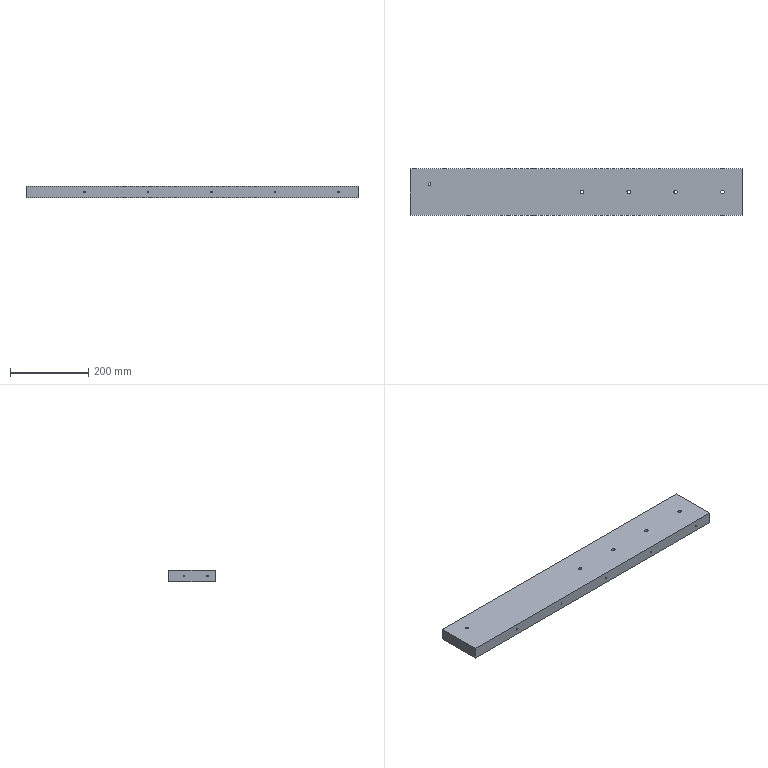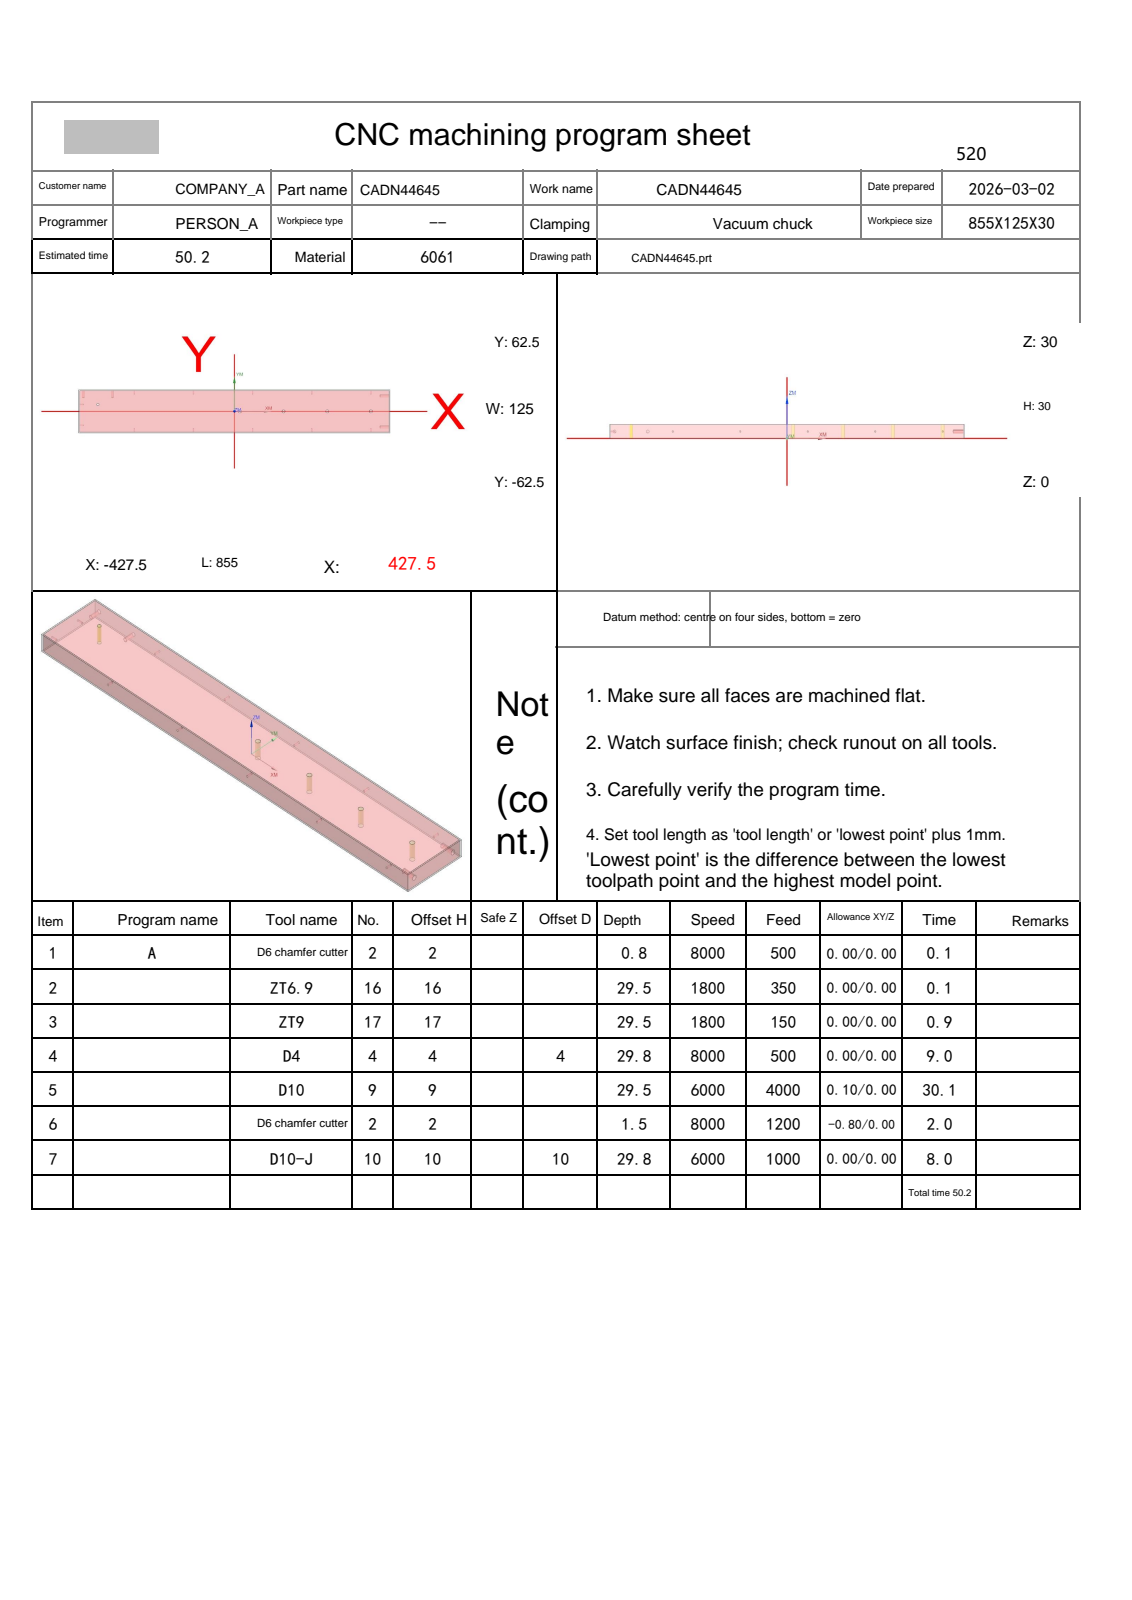NC program | NX | posted by the shop | part box 850 x 120 x 30 mm
Lines 1 to 1477 of 2164, first 1115 of 1475 lines:
%
O0001
(Machine time: 51.65 MIN)
(===Total Tool:6===)
(T2=D6 chamfer cutter   D=6.   R=0.   D-  H02 Z=28.5  )
(T16=ZT6.9  D=6.9  DR_a=120 D-  H16 Z=0.5   )
(T17=ZT9    D=9.   DR_a=118 D-  H17 Z=0.5   )
(T4=D4      D=4.   R=0.   D4  H04 Z=0.2   )
(T9=D10     D=10.  R=0.   D-  H09 Z=0.5   )
(T10=D10-J  D=10.  R=0.   D10 H10 Z=0.2   )
G80 G90 G17 G49 G40
G91 G28 Z0
M01
N1 T02 M06
(D6 chamfer cutter  D=6. R=0. H=02 ce=0.00 di=0.00)
G00 G90 G54 X-375. Y20. M03 S8000
G43 H02 Z80.
M08
G98 G81 X-375. Y20. Z29.2 R31. F500.
X15. Y0.0
X135.
X255.
X375.
G80
G00 Z80.
G91 G28 Z0.0
M05
M09
G91 G28 Z0.0
M01
N2 T16 M06
(ZT6.9 D=6.9 DR_a=120 H=16)
G00 G90 G54 X-375. Y20. M03 S1800
G43 H16 Z80.
M08
G98 G83 X-375. Y20. Z.5 R31. F350. Q3.
G80
G00 Z80.
G91 G28 Z0.0
M05
M09
G91 G28 Z0.0
M01
N3 T17 M06
(ZT9 D=9. DR_a=118 H=17)
G00 G90 G54 X375. Y0.0 M03 S1800
G43 H17 Z80.
M08
G98 G83 X375. Y0.0 Z.5 R31. F150. Q3.
X255.
X135.
X15.
G80
G00 Z80.
G91 G28 Z0.0
M05
M09
G91 G28 Z0.0
M01
N4 T04 M06
(D4  D=4. R=0. H=04 ce=0.00 di=0.00)
G00 G90 G54 X373.18 Y1.661 M03 S8000
G43 H04 Z80.
M08
Z30.5
G01 X373.119 Y1.601 Z30.496 F500.
X372.888 Y1.28 Z30.475
X372.71 Y.926 Z30.454
X372.592 Y.549 Z30.433
X372.535 Y.157 Z30.413
Y-.157 Z30.396
X372.592 Y-.549 Z30.375
X372.71 Y-.926 Z30.355
X372.888 Y-1.28 Z30.334
X373.119 Y-1.601 Z30.313
X373.399 Y-1.881 Z30.292
X373.72 Y-2.112 Z30.272
X374.074 Y-2.29 Z30.251
X374.451 Y-2.408 Z30.23
X374.843 Y-2.465 Z30.209
X375.157 Z30.193
X375.593 Y-2.398 Z30.17
X376.009 Y-2.254 Z30.147
X376.394 Y-2.039 Z30.124
X376.734 Y-1.759 Z30.101
X377.019 Y-1.423 Z30.078
X377.24 Y-1.041 Z30.054
X377.389 Y-.627 Z30.031
X377.462 Y-.192 Z30.008
X377.465 Y-.035 Z30.
G41 D04
X377.5 Y0.0
G03 X375. Y2.5 Z29.876 I-2.5 J0.0
X372.5 Y0.0 Z29.752 I0.0 J-2.5
X375. Y-2.5 Z29.628 I2.5 J0.0
X377.5 Y0.0 Z29.503 I0.0 J2.5
X375. Y2.5 Z29.379 I-2.5 J0.0
X372.5 Y0.0 Z29.255 I0.0 J-2.5
X375. Y-2.5 Z29.131 I2.5 J0.0
X377.5 Y0.0 Z29.007 I0.0 J2.5
X375. Y2.5 Z28.883 I-2.5 J0.0
X372.5 Y0.0 Z28.758 I0.0 J-2.5
X375. Y-2.5 Z28.634 I2.5 J0.0
X377.5 Y0.0 Z28.51 I0.0 J2.5
X375. Y2.5 Z28.386 I-2.5 J0.0
X372.5 Y0.0 Z28.262 I0.0 J-2.5
X375. Y-2.5 Z28.138 I2.5 J0.0
X377.5 Y0.0 Z28.013 I0.0 J2.5
X375. Y2.5 Z27.889 I-2.5 J0.0
X372.5 Y0.0 Z27.765 I0.0 J-2.5
X375. Y-2.5 Z27.641 I2.5 J0.0
X377.5 Y0.0 Z27.517 I0.0 J2.5
X375. Y2.5 Z27.393 I-2.5 J0.0
X372.5 Y0.0 Z27.268 I0.0 J-2.5
X375. Y-2.5 Z27.144 I2.5 J0.0
X377.5 Y0.0 Z27.02 I0.0 J2.5
X375. Y2.5 Z26.896 I-2.5 J0.0
X372.5 Y0.0 Z26.772 I0.0 J-2.5
X375. Y-2.5 Z26.648 I2.5 J0.0
X377.5 Y0.0 Z26.523 I0.0 J2.5
X375. Y2.5 Z26.399 I-2.5 J0.0
X372.5 Y0.0 Z26.275 I0.0 J-2.5
X375. Y-2.5 Z26.151 I2.5 J0.0
X377.5 Y0.0 Z26.027 I0.0 J2.5
X375. Y2.5 Z25.903 I-2.5 J0.0
X372.5 Y0.0 Z25.778 I0.0 J-2.5
X375. Y-2.5 Z25.654 I2.5 J0.0
X377.5 Y0.0 Z25.53 I0.0 J2.5
X375. Y2.5 Z25.406 I-2.5 J0.0
X372.5 Y0.0 Z25.282 I0.0 J-2.5
X375. Y-2.5 Z25.158 I2.5 J0.0
X377.5 Y0.0 Z25.033 I0.0 J2.5
X375. Y2.5 Z24.909 I-2.5 J0.0
X372.5 Y0.0 Z24.785 I0.0 J-2.5
X375. Y-2.5 Z24.661 I2.5 J0.0
X377.5 Y0.0 Z24.537 I0.0 J2.5
X375. Y2.5 Z24.413 I-2.5 J0.0
X372.5 Y0.0 Z24.288 I0.0 J-2.5
X375. Y-2.5 Z24.164 I2.5 J0.0
X377.5 Y0.0 Z24.04 I0.0 J2.5
X375. Y2.5 Z23.916 I-2.5 J0.0
X372.5 Y0.0 Z23.792 I0.0 J-2.5
X375. Y-2.5 Z23.668 I2.5 J0.0
X377.5 Y0.0 Z23.543 I0.0 J2.5
X375. Y2.5 Z23.419 I-2.5 J0.0
X372.5 Y0.0 Z23.295 I0.0 J-2.5
X375. Y-2.5 Z23.171 I2.5 J0.0
X377.5 Y0.0 Z23.047 I0.0 J2.5
X375. Y2.5 Z22.923 I-2.5 J0.0
X372.5 Y0.0 Z22.798 I0.0 J-2.5
X375. Y-2.5 Z22.674 I2.5 J0.0
X377.5 Y0.0 Z22.55 I0.0 J2.5
X375. Y2.5 Z22.426 I-2.5 J0.0
X372.5 Y0.0 Z22.302 I0.0 J-2.5
X375. Y-2.5 Z22.178 I2.5 J0.0
X377.5 Y0.0 Z22.053 I0.0 J2.5
X375. Y2.5 Z21.929 I-2.5 J0.0
X372.5 Y0.0 Z21.805 I0.0 J-2.5
X375. Y-2.5 Z21.681 I2.5 J0.0
X377.5 Y0.0 Z21.557 I0.0 J2.5
X375. Y2.5 Z21.433 I-2.5 J0.0
X372.5 Y0.0 Z21.308 I0.0 J-2.5
X375. Y-2.5 Z21.184 I2.5 J0.0
X377.5 Y0.0 Z21.06 I0.0 J2.5
X375. Y2.5 Z20.936 I-2.5 J0.0
X372.5 Y0.0 Z20.812 I0.0 J-2.5
X375. Y-2.5 Z20.688 I2.5 J0.0
X377.5 Y0.0 Z20.563 I0.0 J2.5
X375. Y2.5 Z20.439 I-2.5 J0.0
X372.5 Y0.0 Z20.315 I0.0 J-2.5
X375. Y-2.5 Z20.191 I2.5 J0.0
X377.5 Y0.0 Z20.067 I0.0 J2.5
X375. Y2.5 Z19.943 I-2.5 J0.0
X372.5 Y0.0 Z19.818 I0.0 J-2.5
X375. Y-2.5 Z19.694 I2.5 J0.0
X377.5 Y0.0 Z19.57 I0.0 J2.5
X375. Y2.5 Z19.446 I-2.5 J0.0
X372.5 Y0.0 Z19.322 I0.0 J-2.5
X375. Y-2.5 Z19.198 I2.5 J0.0
X377.5 Y0.0 Z19.073 I0.0 J2.5
X375. Y2.5 Z18.949 I-2.5 J0.0
X372.5 Y0.0 Z18.825 I0.0 J-2.5
X375. Y-2.5 Z18.701 I2.5 J0.0
X377.5 Y0.0 Z18.577 I0.0 J2.5
X375. Y2.5 Z18.453 I-2.5 J0.0
X372.5 Y0.0 Z18.328 I0.0 J-2.5
X375. Y-2.5 Z18.204 I2.5 J0.0
X377.5 Y0.0 Z18.08 I0.0 J2.5
X375. Y2.5 Z17.956 I-2.5 J0.0
X372.5 Y0.0 Z17.832 I0.0 J-2.5
X375. Y-2.5 Z17.708 I2.5 J0.0
X377.5 Y0.0 Z17.583 I0.0 J2.5
X375. Y2.5 Z17.459 I-2.5 J0.0
X372.5 Y0.0 Z17.335 I0.0 J-2.5
X375. Y-2.5 Z17.211 I2.5 J0.0
X377.5 Y0.0 Z17.087 I0.0 J2.5
X375. Y2.5 Z16.963 I-2.5 J0.0
X372.5 Y0.0 Z16.838 I0.0 J-2.5
X375. Y-2.5 Z16.714 I2.5 J0.0
X377.5 Y0.0 Z16.59 I0.0 J2.5
X375. Y2.5 Z16.466 I-2.5 J0.0
X372.5 Y0.0 Z16.342 I0.0 J-2.5
X375. Y-2.5 Z16.218 I2.5 J0.0
X377.5 Y0.0 Z16.093 I0.0 J2.5
X375. Y2.5 Z15.969 I-2.5 J0.0
X372.5 Y0.0 Z15.845 I0.0 J-2.5
X375. Y-2.5 Z15.721 I2.5 J0.0
X377.5 Y0.0 Z15.597 I0.0 J2.5
X375. Y2.5 Z15.473 I-2.5 J0.0
X372.5 Y0.0 Z15.348 I0.0 J-2.5
X375. Y-2.5 Z15.224 I2.5 J0.0
X377.5 Y0.0 Z15.1 I0.0 J2.5
X375. Y2.5 Z14.976 I-2.5 J0.0
X372.5 Y0.0 Z14.852 I0.0 J-2.5
X375. Y-2.5 Z14.728 I2.5 J0.0
X377.5 Y0.0 Z14.603 I0.0 J2.5
X375. Y2.5 Z14.479 I-2.5 J0.0
X372.5 Y0.0 Z14.355 I0.0 J-2.5
X375. Y-2.5 Z14.231 I2.5 J0.0
X377.5 Y0.0 Z14.107 I0.0 J2.5
X375. Y2.5 Z13.983 I-2.5 J0.0
X372.5 Y0.0 Z13.858 I0.0 J-2.5
X375. Y-2.5 Z13.734 I2.5 J0.0
X377.5 Y0.0 Z13.61 I0.0 J2.5
X375. Y2.5 Z13.486 I-2.5 J0.0
X372.5 Y0.0 Z13.362 I0.0 J-2.5
X375. Y-2.5 Z13.238 I2.5 J0.0
X377.5 Y0.0 Z13.113 I0.0 J2.5
X375. Y2.5 Z12.989 I-2.5 J0.0
X372.5 Y0.0 Z12.865 I0.0 J-2.5
X375. Y-2.5 Z12.741 I2.5 J0.0
X377.5 Y0.0 Z12.617 I0.0 J2.5
X375. Y2.5 Z12.493 I-2.5 J0.0
X372.5 Y0.0 Z12.368 I0.0 J-2.5
X375. Y-2.5 Z12.244 I2.5 J0.0
X377.5 Y0.0 Z12.12 I0.0 J2.5
X375. Y2.5 Z11.996 I-2.5 J0.0
X372.5 Y0.0 Z11.872 I0.0 J-2.5
X375. Y-2.5 Z11.748 I2.5 J0.0
X377.5 Y0.0 Z11.623 I0.0 J2.5
X375. Y2.5 Z11.499 I-2.5 J0.0
X372.5 Y0.0 Z11.375 I0.0 J-2.5
X375. Y-2.5 Z11.251 I2.5 J0.0
X377.5 Y0.0 Z11.127 I0.0 J2.5
X375. Y2.5 Z11.003 I-2.5 J0.0
X372.5 Y0.0 Z10.878 I0.0 J-2.5
X375. Y-2.5 Z10.754 I2.5 J0.0
X377.5 Y0.0 Z10.63 I0.0 J2.5
X375. Y2.5 Z10.506 I-2.5 J0.0
X372.5 Y0.0 Z10.382 I0.0 J-2.5
X375. Y-2.5 Z10.258 I2.5 J0.0
X377.5 Y0.0 Z10.133 I0.0 J2.5
X375. Y2.5 Z10.009 I-2.5 J0.0
X372.5 Y0.0 Z9.885 I0.0 J-2.5
X375. Y-2.5 Z9.761 I2.5 J0.0
X377.5 Y0.0 Z9.637 I0.0 J2.5
X375. Y2.5 Z9.513 I-2.5 J0.0
X372.5 Y0.0 Z9.388 I0.0 J-2.5
X375. Y-2.5 Z9.264 I2.5 J0.0
X377.5 Y0.0 Z9.14 I0.0 J2.5
X375. Y2.5 Z9.016 I-2.5 J0.0
X372.5 Y0.0 Z8.892 I0.0 J-2.5
X375. Y-2.5 Z8.768 I2.5 J0.0
X377.5 Y0.0 Z8.643 I0.0 J2.5
X375. Y2.5 Z8.519 I-2.5 J0.0
X372.5 Y0.0 Z8.395 I0.0 J-2.5
X375. Y-2.5 Z8.271 I2.5 J0.0
X377.5 Y0.0 Z8.147 I0.0 J2.5
X375. Y2.5 Z8.023 I-2.5 J0.0
X372.5 Y0.0 Z7.898 I0.0 J-2.5
X375. Y-2.5 Z7.774 I2.5 J0.0
X377.5 Y0.0 Z7.65 I0.0 J2.5
X375. Y2.5 Z7.526 I-2.5 J0.0
X372.5 Y0.0 Z7.402 I0.0 J-2.5
X375. Y-2.5 Z7.278 I2.5 J0.0
X377.5 Y0.0 Z7.153 I0.0 J2.5
X375. Y2.5 Z7.029 I-2.5 J0.0
X372.5 Y0.0 Z6.905 I0.0 J-2.5
X375. Y-2.5 Z6.781 I2.5 J0.0
X377.5 Y0.0 Z6.657 I0.0 J2.5
X375. Y2.5 Z6.533 I-2.5 J0.0
X372.5 Y0.0 Z6.408 I0.0 J-2.5
X375. Y-2.5 Z6.284 I2.5 J0.0
X377.5 Y0.0 Z6.16 I0.0 J2.5
X375. Y2.5 Z6.036 I-2.5 J0.0
X372.5 Y0.0 Z5.912 I0.0 J-2.5
X375. Y-2.5 Z5.788 I2.5 J0.0
X377.5 Y0.0 Z5.663 I0.0 J2.5
X375. Y2.5 Z5.539 I-2.5 J0.0
X372.5 Y0.0 Z5.415 I0.0 J-2.5
X375. Y-2.5 Z5.291 I2.5 J0.0
X377.5 Y0.0 Z5.167 I0.0 J2.5
X375. Y2.5 Z5.043 I-2.5 J0.0
X372.5 Y0.0 Z4.918 I0.0 J-2.5
X375. Y-2.5 Z4.794 I2.5 J0.0
X377.5 Y0.0 Z4.67 I0.0 J2.5
X375. Y2.5 Z4.546 I-2.5 J0.0
X372.5 Y0.0 Z4.422 I0.0 J-2.5
X375. Y-2.5 Z4.298 I2.5 J0.0
X377.5 Y0.0 Z4.173 I0.0 J2.5
X375. Y2.5 Z4.049 I-2.5 J0.0
X372.5 Y0.0 Z3.925 I0.0 J-2.5
X375. Y-2.5 Z3.801 I2.5 J0.0
X377.5 Y0.0 Z3.677 I0.0 J2.5
X375. Y2.5 Z3.553 I-2.5 J0.0
X372.5 Y0.0 Z3.428 I0.0 J-2.5
X375. Y-2.5 Z3.304 I2.5 J0.0
X377.5 Y0.0 Z3.18 I0.0 J2.5
X375. Y2.5 Z3.056 I-2.5 J0.0
X372.5 Y0.0 Z2.932 I0.0 J-2.5
X375. Y-2.5 Z2.808 I2.5 J0.0
X377.5 Y0.0 Z2.683 I0.0 J2.5
X375. Y2.5 Z2.559 I-2.5 J0.0
X372.5 Y0.0 Z2.435 I0.0 J-2.5
X375. Y-2.5 Z2.311 I2.5 J0.0
X377.5 Y0.0 Z2.187 I0.0 J2.5
X375. Y2.5 Z2.063 I-2.5 J0.0
X372.5 Y0.0 Z1.938 I0.0 J-2.5
X375. Y-2.5 Z1.814 I2.5 J0.0
X377.5 Y0.0 Z1.69 I0.0 J2.5
X375. Y2.5 Z1.566 I-2.5 J0.0
X372.5 Y0.0 Z1.442 I0.0 J-2.5
X375. Y-2.5 Z1.318 I2.5 J0.0
X377.5 Y0.0 Z1.193 I0.0 J2.5
X375. Y2.5 Z1.069 I-2.5 J0.0
X372.5 Y0.0 Z.945 I0.0 J-2.5
X375. Y-2.5 Z.821 I2.5 J0.0
X377.5 Y0.0 Z.697 I0.0 J2.5
X375. Y2.5 Z.573 I-2.5 J0.0
X372.5 Y0.0 Z.448 I0.0 J-2.5
X375. Y-2.5 Z.324 I2.5 J0.0
X377.5 Y0.0 Z.2 I0.0 J2.5
X375. Y2.5 I-2.5 J0.0
X372.5 Y0.0 I0.0 J-2.5
X375. Y-2.5 I2.5 J0.0
X377.5 Y0.0 I0.0 J2.5
X377.468 Y.398 I-2.5 J0.0
G01 X377.461 Y.425
X377.438 Y.442
X377.411 Y.44
G40 X377.361 Y.432
Z1.2
G00 Z80.
X256.661 Y1.82
Z30.5
G01 X256.601 Y1.881 Z30.496
X256.28 Y2.112 Z30.475
X255.926 Y2.29 Z30.454
X255.549 Y2.408 Z30.433
X255.157 Y2.465 Z30.413
X254.843 Z30.396
X254.451 Y2.408 Z30.375
X254.074 Y2.29 Z30.355
X253.72 Y2.112 Z30.334
X253.399 Y1.881 Z30.313
X253.119 Y1.601 Z30.292
X252.888 Y1.28 Z30.272
X252.71 Y.926 Z30.251
X252.592 Y.549 Z30.23
X252.535 Y.157 Z30.209
Y-.157 Z30.193
X252.602 Y-.593 Z30.17
X252.746 Y-1.009 Z30.147
X252.961 Y-1.394 Z30.124
X253.241 Y-1.734 Z30.101
X253.577 Y-2.019 Z30.078
X253.959 Y-2.24 Z30.054
X254.373 Y-2.389 Z30.031
X254.808 Y-2.462 Z30.008
X254.965 Y-2.465 Z30.
G41 D04
X255. Y-2.5
G03 X257.5 Y0.0 Z29.876 I0.0 J2.5
X255. Y2.5 Z29.752 I-2.5 J0.0
X252.5 Y0.0 Z29.628 I0.0 J-2.5
X255. Y-2.5 Z29.503 I2.5 J0.0
X257.5 Y0.0 Z29.379 I0.0 J2.5
X255. Y2.5 Z29.255 I-2.5 J0.0
X252.5 Y0.0 Z29.131 I0.0 J-2.5
X255. Y-2.5 Z29.007 I2.5 J0.0
X257.5 Y0.0 Z28.883 I0.0 J2.5
X255. Y2.5 Z28.758 I-2.5 J0.0
X252.5 Y0.0 Z28.634 I0.0 J-2.5
X255. Y-2.5 Z28.51 I2.5 J0.0
X257.5 Y0.0 Z28.386 I0.0 J2.5
X255. Y2.5 Z28.262 I-2.5 J0.0
X252.5 Y0.0 Z28.138 I0.0 J-2.5
X255. Y-2.5 Z28.013 I2.5 J0.0
X257.5 Y0.0 Z27.889 I0.0 J2.5
X255. Y2.5 Z27.765 I-2.5 J0.0
X252.5 Y0.0 Z27.641 I0.0 J-2.5
X255. Y-2.5 Z27.517 I2.5 J0.0
X257.5 Y0.0 Z27.393 I0.0 J2.5
X255. Y2.5 Z27.268 I-2.5 J0.0
X252.5 Y0.0 Z27.144 I0.0 J-2.5
X255. Y-2.5 Z27.02 I2.5 J0.0
X257.5 Y0.0 Z26.896 I0.0 J2.5
X255. Y2.5 Z26.772 I-2.5 J0.0
X252.5 Y0.0 Z26.648 I0.0 J-2.5
X255. Y-2.5 Z26.523 I2.5 J0.0
X257.5 Y0.0 Z26.399 I0.0 J2.5
X255. Y2.5 Z26.275 I-2.5 J0.0
X252.5 Y0.0 Z26.151 I0.0 J-2.5
X255. Y-2.5 Z26.027 I2.5 J0.0
X257.5 Y0.0 Z25.903 I0.0 J2.5
X255. Y2.5 Z25.778 I-2.5 J0.0
X252.5 Y0.0 Z25.654 I0.0 J-2.5
X255. Y-2.5 Z25.53 I2.5 J0.0
X257.5 Y0.0 Z25.406 I0.0 J2.5
X255. Y2.5 Z25.282 I-2.5 J0.0
X252.5 Y0.0 Z25.158 I0.0 J-2.5
X255. Y-2.5 Z25.033 I2.5 J0.0
X257.5 Y0.0 Z24.909 I0.0 J2.5
X255. Y2.5 Z24.785 I-2.5 J0.0
X252.5 Y0.0 Z24.661 I0.0 J-2.5
X255. Y-2.5 Z24.537 I2.5 J0.0
X257.5 Y0.0 Z24.413 I0.0 J2.5
X255. Y2.5 Z24.288 I-2.5 J0.0
X252.5 Y0.0 Z24.164 I0.0 J-2.5
X255. Y-2.5 Z24.04 I2.5 J0.0
X257.5 Y0.0 Z23.916 I0.0 J2.5
X255. Y2.5 Z23.792 I-2.5 J0.0
X252.5 Y0.0 Z23.668 I0.0 J-2.5
X255. Y-2.5 Z23.543 I2.5 J0.0
X257.5 Y0.0 Z23.419 I0.0 J2.5
X255. Y2.5 Z23.295 I-2.5 J0.0
X252.5 Y0.0 Z23.171 I0.0 J-2.5
X255. Y-2.5 Z23.047 I2.5 J0.0
X257.5 Y0.0 Z22.923 I0.0 J2.5
X255. Y2.5 Z22.798 I-2.5 J0.0
X252.5 Y0.0 Z22.674 I0.0 J-2.5
X255. Y-2.5 Z22.55 I2.5 J0.0
X257.5 Y0.0 Z22.426 I0.0 J2.5
X255. Y2.5 Z22.302 I-2.5 J0.0
X252.5 Y0.0 Z22.178 I0.0 J-2.5
X255. Y-2.5 Z22.053 I2.5 J0.0
X257.5 Y0.0 Z21.929 I0.0 J2.5
X255. Y2.5 Z21.805 I-2.5 J0.0
X252.5 Y0.0 Z21.681 I0.0 J-2.5
X255. Y-2.5 Z21.557 I2.5 J0.0
X257.5 Y0.0 Z21.433 I0.0 J2.5
X255. Y2.5 Z21.308 I-2.5 J0.0
X252.5 Y0.0 Z21.184 I0.0 J-2.5
X255. Y-2.5 Z21.06 I2.5 J0.0
X257.5 Y0.0 Z20.936 I0.0 J2.5
X255. Y2.5 Z20.812 I-2.5 J0.0
X252.5 Y0.0 Z20.688 I0.0 J-2.5
X255. Y-2.5 Z20.563 I2.5 J0.0
X257.5 Y0.0 Z20.439 I0.0 J2.5
X255. Y2.5 Z20.315 I-2.5 J0.0
X252.5 Y0.0 Z20.191 I0.0 J-2.5
X255. Y-2.5 Z20.067 I2.5 J0.0
X257.5 Y0.0 Z19.943 I0.0 J2.5
X255. Y2.5 Z19.818 I-2.5 J0.0
X252.5 Y0.0 Z19.694 I0.0 J-2.5
X255. Y-2.5 Z19.57 I2.5 J0.0
X257.5 Y0.0 Z19.446 I0.0 J2.5
X255. Y2.5 Z19.322 I-2.5 J0.0
X252.5 Y0.0 Z19.198 I0.0 J-2.5
X255. Y-2.5 Z19.073 I2.5 J0.0
X257.5 Y0.0 Z18.949 I0.0 J2.5
X255. Y2.5 Z18.825 I-2.5 J0.0
X252.5 Y0.0 Z18.701 I0.0 J-2.5
X255. Y-2.5 Z18.577 I2.5 J0.0
X257.5 Y0.0 Z18.453 I0.0 J2.5
X255. Y2.5 Z18.328 I-2.5 J0.0
X252.5 Y0.0 Z18.204 I0.0 J-2.5
X255. Y-2.5 Z18.08 I2.5 J0.0
X257.5 Y0.0 Z17.956 I0.0 J2.5
X255. Y2.5 Z17.832 I-2.5 J0.0
X252.5 Y0.0 Z17.708 I0.0 J-2.5
X255. Y-2.5 Z17.583 I2.5 J0.0
X257.5 Y0.0 Z17.459 I0.0 J2.5
X255. Y2.5 Z17.335 I-2.5 J0.0
X252.5 Y0.0 Z17.211 I0.0 J-2.5
X255. Y-2.5 Z17.087 I2.5 J0.0
X257.5 Y0.0 Z16.963 I0.0 J2.5
X255. Y2.5 Z16.838 I-2.5 J0.0
X252.5 Y0.0 Z16.714 I0.0 J-2.5
X255. Y-2.5 Z16.59 I2.5 J0.0
X257.5 Y0.0 Z16.466 I0.0 J2.5
X255. Y2.5 Z16.342 I-2.5 J0.0
X252.5 Y0.0 Z16.218 I0.0 J-2.5
X255. Y-2.5 Z16.093 I2.5 J0.0
X257.5 Y0.0 Z15.969 I0.0 J2.5
X255. Y2.5 Z15.845 I-2.5 J0.0
X252.5 Y0.0 Z15.721 I0.0 J-2.5
X255. Y-2.5 Z15.597 I2.5 J0.0
X257.5 Y0.0 Z15.473 I0.0 J2.5
X255. Y2.5 Z15.348 I-2.5 J0.0
X252.5 Y0.0 Z15.224 I0.0 J-2.5
X255. Y-2.5 Z15.1 I2.5 J0.0
X257.5 Y0.0 Z14.976 I0.0 J2.5
X255. Y2.5 Z14.852 I-2.5 J0.0
X252.5 Y0.0 Z14.728 I0.0 J-2.5
X255. Y-2.5 Z14.603 I2.5 J0.0
X257.5 Y0.0 Z14.479 I0.0 J2.5
X255. Y2.5 Z14.355 I-2.5 J0.0
X252.5 Y0.0 Z14.231 I0.0 J-2.5
X255. Y-2.5 Z14.107 I2.5 J0.0
X257.5 Y0.0 Z13.983 I0.0 J2.5
X255. Y2.5 Z13.858 I-2.5 J0.0
X252.5 Y0.0 Z13.734 I0.0 J-2.5
X255. Y-2.5 Z13.61 I2.5 J0.0
X257.5 Y0.0 Z13.486 I0.0 J2.5
X255. Y2.5 Z13.362 I-2.5 J0.0
X252.5 Y0.0 Z13.238 I0.0 J-2.5
X255. Y-2.5 Z13.113 I2.5 J0.0
X257.5 Y0.0 Z12.989 I0.0 J2.5
X255. Y2.5 Z12.865 I-2.5 J0.0
X252.5 Y0.0 Z12.741 I0.0 J-2.5
X255. Y-2.5 Z12.617 I2.5 J0.0
X257.5 Y0.0 Z12.493 I0.0 J2.5
X255. Y2.5 Z12.368 I-2.5 J0.0
X252.5 Y0.0 Z12.244 I0.0 J-2.5
X255. Y-2.5 Z12.12 I2.5 J0.0
X257.5 Y0.0 Z11.996 I0.0 J2.5
X255. Y2.5 Z11.872 I-2.5 J0.0
X252.5 Y0.0 Z11.748 I0.0 J-2.5
X255. Y-2.5 Z11.623 I2.5 J0.0
X257.5 Y0.0 Z11.499 I0.0 J2.5
X255. Y2.5 Z11.375 I-2.5 J0.0
X252.5 Y0.0 Z11.251 I0.0 J-2.5
X255. Y-2.5 Z11.127 I2.5 J0.0
X257.5 Y0.0 Z11.003 I0.0 J2.5
X255. Y2.5 Z10.878 I-2.5 J0.0
X252.5 Y0.0 Z10.754 I0.0 J-2.5
X255. Y-2.5 Z10.63 I2.5 J0.0
X257.5 Y0.0 Z10.506 I0.0 J2.5
X255. Y2.5 Z10.382 I-2.5 J0.0
X252.5 Y0.0 Z10.258 I0.0 J-2.5
X255. Y-2.5 Z10.133 I2.5 J0.0
X257.5 Y0.0 Z10.009 I0.0 J2.5
X255. Y2.5 Z9.885 I-2.5 J0.0
X252.5 Y0.0 Z9.761 I0.0 J-2.5
X255. Y-2.5 Z9.637 I2.5 J0.0
X257.5 Y0.0 Z9.513 I0.0 J2.5
X255. Y2.5 Z9.388 I-2.5 J0.0
X252.5 Y0.0 Z9.264 I0.0 J-2.5
X255. Y-2.5 Z9.14 I2.5 J0.0
X257.5 Y0.0 Z9.016 I0.0 J2.5
X255. Y2.5 Z8.892 I-2.5 J0.0
X252.5 Y0.0 Z8.768 I0.0 J-2.5
X255. Y-2.5 Z8.643 I2.5 J0.0
X257.5 Y0.0 Z8.519 I0.0 J2.5
X255. Y2.5 Z8.395 I-2.5 J0.0
X252.5 Y0.0 Z8.271 I0.0 J-2.5
X255. Y-2.5 Z8.147 I2.5 J0.0
X257.5 Y0.0 Z8.023 I0.0 J2.5
X255. Y2.5 Z7.898 I-2.5 J0.0
X252.5 Y0.0 Z7.774 I0.0 J-2.5
X255. Y-2.5 Z7.65 I2.5 J0.0
X257.5 Y0.0 Z7.526 I0.0 J2.5
X255. Y2.5 Z7.402 I-2.5 J0.0
X252.5 Y0.0 Z7.278 I0.0 J-2.5
X255. Y-2.5 Z7.153 I2.5 J0.0
X257.5 Y0.0 Z7.029 I0.0 J2.5
X255. Y2.5 Z6.905 I-2.5 J0.0
X252.5 Y0.0 Z6.781 I0.0 J-2.5
X255. Y-2.5 Z6.657 I2.5 J0.0
X257.5 Y0.0 Z6.533 I0.0 J2.5
X255. Y2.5 Z6.408 I-2.5 J0.0
X252.5 Y0.0 Z6.284 I0.0 J-2.5
X255. Y-2.5 Z6.16 I2.5 J0.0
X257.5 Y0.0 Z6.036 I0.0 J2.5
X255. Y2.5 Z5.912 I-2.5 J0.0
X252.5 Y0.0 Z5.788 I0.0 J-2.5
X255. Y-2.5 Z5.663 I2.5 J0.0
X257.5 Y0.0 Z5.539 I0.0 J2.5
X255. Y2.5 Z5.415 I-2.5 J0.0
X252.5 Y0.0 Z5.291 I0.0 J-2.5
X255. Y-2.5 Z5.167 I2.5 J0.0
X257.5 Y0.0 Z5.043 I0.0 J2.5
X255. Y2.5 Z4.918 I-2.5 J0.0
X252.5 Y0.0 Z4.794 I0.0 J-2.5
X255. Y-2.5 Z4.67 I2.5 J0.0
X257.5 Y0.0 Z4.546 I0.0 J2.5
X255. Y2.5 Z4.422 I-2.5 J0.0
X252.5 Y0.0 Z4.298 I0.0 J-2.5
X255. Y-2.5 Z4.173 I2.5 J0.0
X257.5 Y0.0 Z4.049 I0.0 J2.5
X255. Y2.5 Z3.925 I-2.5 J0.0
X252.5 Y0.0 Z3.801 I0.0 J-2.5
X255. Y-2.5 Z3.677 I2.5 J0.0
X257.5 Y0.0 Z3.553 I0.0 J2.5
X255. Y2.5 Z3.428 I-2.5 J0.0
X252.5 Y0.0 Z3.304 I0.0 J-2.5
X255. Y-2.5 Z3.18 I2.5 J0.0
X257.5 Y0.0 Z3.056 I0.0 J2.5
X255. Y2.5 Z2.932 I-2.5 J0.0
X252.5 Y0.0 Z2.808 I0.0 J-2.5
X255. Y-2.5 Z2.683 I2.5 J0.0
X257.5 Y0.0 Z2.559 I0.0 J2.5
X255. Y2.5 Z2.435 I-2.5 J0.0
X252.5 Y0.0 Z2.311 I0.0 J-2.5
X255. Y-2.5 Z2.187 I2.5 J0.0
X257.5 Y0.0 Z2.063 I0.0 J2.5
X255. Y2.5 Z1.938 I-2.5 J0.0
X252.5 Y0.0 Z1.814 I0.0 J-2.5
X255. Y-2.5 Z1.69 I2.5 J0.0
X257.5 Y0.0 Z1.566 I0.0 J2.5
X255. Y2.5 Z1.442 I-2.5 J0.0
X252.5 Y0.0 Z1.318 I0.0 J-2.5
X255. Y-2.5 Z1.193 I2.5 J0.0
X257.5 Y0.0 Z1.069 I0.0 J2.5
X255. Y2.5 Z.945 I-2.5 J0.0
X252.5 Y0.0 Z.821 I0.0 J-2.5
X255. Y-2.5 Z.697 I2.5 J0.0
X257.5 Y0.0 Z.573 I0.0 J2.5
X255. Y2.5 Z.448 I-2.5 J0.0
X252.5 Y0.0 Z.324 I0.0 J-2.5
X255. Y-2.5 Z.2 I2.5 J0.0
X257.5 Y0.0 I0.0 J2.5
X255. Y2.5 I-2.5 J0.0
X252.5 Y0.0 I0.0 J-2.5
X255. Y-2.5 I2.5 J0.0
X255.398 Y-2.468 I0.0 J2.5
G01 X255.425 Y-2.461
X255.442 Y-2.438
X255.44 Y-2.411
G40 X255.432 Y-2.361
Z1.2
G00 Z80.
X136.661 Y1.82
Z30.5
G01 X136.601 Y1.881 Z30.496
X136.28 Y2.112 Z30.475
X135.926 Y2.29 Z30.454
X135.549 Y2.408 Z30.433
X135.157 Y2.465 Z30.413
X134.843 Z30.396
X134.451 Y2.408 Z30.375
X134.074 Y2.29 Z30.355
X133.72 Y2.112 Z30.334
X133.399 Y1.881 Z30.313
X133.119 Y1.601 Z30.292
X132.888 Y1.28 Z30.272
X132.71 Y.926 Z30.251
X132.592 Y.549 Z30.23
X132.535 Y.157 Z30.209
Y-.157 Z30.193
X132.602 Y-.593 Z30.17
X132.746 Y-1.009 Z30.147
X132.961 Y-1.394 Z30.124
X133.241 Y-1.734 Z30.101
X133.577 Y-2.019 Z30.078
X133.959 Y-2.24 Z30.054
X134.373 Y-2.389 Z30.031
X134.808 Y-2.462 Z30.008
X134.965 Y-2.465 Z30.
G41 D04
X135. Y-2.5
G03 X137.5 Y0.0 Z29.876 I0.0 J2.5
X135. Y2.5 Z29.752 I-2.5 J0.0
X132.5 Y0.0 Z29.628 I0.0 J-2.5
X135. Y-2.5 Z29.503 I2.5 J0.0
X137.5 Y0.0 Z29.379 I0.0 J2.5
X135. Y2.5 Z29.255 I-2.5 J0.0
X132.5 Y0.0 Z29.131 I0.0 J-2.5
X135. Y-2.5 Z29.007 I2.5 J0.0
X137.5 Y0.0 Z28.883 I0.0 J2.5
X135. Y2.5 Z28.758 I-2.5 J0.0
X132.5 Y0.0 Z28.634 I0.0 J-2.5
X135. Y-2.5 Z28.51 I2.5 J0.0
X137.5 Y0.0 Z28.386 I0.0 J2.5
X135. Y2.5 Z28.262 I-2.5 J0.0
X132.5 Y0.0 Z28.138 I0.0 J-2.5
X135. Y-2.5 Z28.013 I2.5 J0.0
X137.5 Y0.0 Z27.889 I0.0 J2.5
X135. Y2.5 Z27.765 I-2.5 J0.0
X132.5 Y0.0 Z27.641 I0.0 J-2.5
X135. Y-2.5 Z27.517 I2.5 J0.0
X137.5 Y0.0 Z27.393 I0.0 J2.5
X135. Y2.5 Z27.268 I-2.5 J0.0
X132.5 Y0.0 Z27.144 I0.0 J-2.5
X135. Y-2.5 Z27.02 I2.5 J0.0
X137.5 Y0.0 Z26.896 I0.0 J2.5
X135. Y2.5 Z26.772 I-2.5 J0.0
X132.5 Y0.0 Z26.648 I0.0 J-2.5
X135. Y-2.5 Z26.523 I2.5 J0.0
X137.5 Y0.0 Z26.399 I0.0 J2.5
X135. Y2.5 Z26.275 I-2.5 J0.0
X132.5 Y0.0 Z26.151 I0.0 J-2.5
X135. Y-2.5 Z26.027 I2.5 J0.0
X137.5 Y0.0 Z25.903 I0.0 J2.5
X135. Y2.5 Z25.778 I-2.5 J0.0
X132.5 Y0.0 Z25.654 I0.0 J-2.5
X135. Y-2.5 Z25.53 I2.5 J0.0
X137.5 Y0.0 Z25.406 I0.0 J2.5
X135. Y2.5 Z25.282 I-2.5 J0.0
X132.5 Y0.0 Z25.158 I0.0 J-2.5
X135. Y-2.5 Z25.033 I2.5 J0.0
X137.5 Y0.0 Z24.909 I0.0 J2.5
X135. Y2.5 Z24.785 I-2.5 J0.0
X132.5 Y0.0 Z24.661 I0.0 J-2.5
X135. Y-2.5 Z24.537 I2.5 J0.0
X137.5 Y0.0 Z24.413 I0.0 J2.5
X135. Y2.5 Z24.288 I-2.5 J0.0
X132.5 Y0.0 Z24.164 I0.0 J-2.5
X135. Y-2.5 Z24.04 I2.5 J0.0
X137.5 Y0.0 Z23.916 I0.0 J2.5
X135. Y2.5 Z23.792 I-2.5 J0.0
X132.5 Y0.0 Z23.668 I0.0 J-2.5
X135. Y-2.5 Z23.543 I2.5 J0.0
X137.5 Y0.0 Z23.419 I0.0 J2.5
X135. Y2.5 Z23.295 I-2.5 J0.0
X132.5 Y0.0 Z23.171 I0.0 J-2.5
X135. Y-2.5 Z23.047 I2.5 J0.0
X137.5 Y0.0 Z22.923 I0.0 J2.5
X135. Y2.5 Z22.798 I-2.5 J0.0
X132.5 Y0.0 Z22.674 I0.0 J-2.5
X135. Y-2.5 Z22.55 I2.5 J0.0
X137.5 Y0.0 Z22.426 I0.0 J2.5
X135. Y2.5 Z22.302 I-2.5 J0.0
X132.5 Y0.0 Z22.178 I0.0 J-2.5
X135. Y-2.5 Z22.053 I2.5 J0.0
X137.5 Y0.0 Z21.929 I0.0 J2.5
X135. Y2.5 Z21.805 I-2.5 J0.0
X132.5 Y0.0 Z21.681 I0.0 J-2.5
X135. Y-2.5 Z21.557 I2.5 J0.0
X137.5 Y0.0 Z21.433 I0.0 J2.5
X135. Y2.5 Z21.308 I-2.5 J0.0
X132.5 Y0.0 Z21.184 I0.0 J-2.5
X135. Y-2.5 Z21.06 I2.5 J0.0
X137.5 Y0.0 Z20.936 I0.0 J2.5
X135. Y2.5 Z20.812 I-2.5 J0.0
X132.5 Y0.0 Z20.688 I0.0 J-2.5
X135. Y-2.5 Z20.563 I2.5 J0.0
X137.5 Y0.0 Z20.439 I0.0 J2.5
X135. Y2.5 Z20.315 I-2.5 J0.0
X132.5 Y0.0 Z20.191 I0.0 J-2.5
X135. Y-2.5 Z20.067 I2.5 J0.0
X137.5 Y0.0 Z19.943 I0.0 J2.5
X135. Y2.5 Z19.818 I-2.5 J0.0
X132.5 Y0.0 Z19.694 I0.0 J-2.5
X135. Y-2.5 Z19.57 I2.5 J0.0
X137.5 Y0.0 Z19.446 I0.0 J2.5
X135. Y2.5 Z19.322 I-2.5 J0.0
X132.5 Y0.0 Z19.198 I0.0 J-2.5
X135. Y-2.5 Z19.073 I2.5 J0.0
X137.5 Y0.0 Z18.949 I0.0 J2.5
X135. Y2.5 Z18.825 I-2.5 J0.0
X132.5 Y0.0 Z18.701 I0.0 J-2.5
X135. Y-2.5 Z18.577 I2.5 J0.0
X137.5 Y0.0 Z18.453 I0.0 J2.5
X135. Y2.5 Z18.328 I-2.5 J0.0
X132.5 Y0.0 Z18.204 I0.0 J-2.5
X135. Y-2.5 Z18.08 I2.5 J0.0
X137.5 Y0.0 Z17.956 I0.0 J2.5
X135. Y2.5 Z17.832 I-2.5 J0.0
X132.5 Y0.0 Z17.708 I0.0 J-2.5
X135. Y-2.5 Z17.583 I2.5 J0.0
X137.5 Y0.0 Z17.459 I0.0 J2.5
X135. Y2.5 Z17.335 I-2.5 J0.0
X132.5 Y0.0 Z17.211 I0.0 J-2.5
X135. Y-2.5 Z17.087 I2.5 J0.0
X137.5 Y0.0 Z16.963 I0.0 J2.5
X135. Y2.5 Z16.838 I-2.5 J0.0
X132.5 Y0.0 Z16.714 I0.0 J-2.5
X135. Y-2.5 Z16.59 I2.5 J0.0
X137.5 Y0.0 Z16.466 I0.0 J2.5
X135. Y2.5 Z16.342 I-2.5 J0.0
X132.5 Y0.0 Z16.218 I0.0 J-2.5
X135. Y-2.5 Z16.093 I2.5 J0.0
X137.5 Y0.0 Z15.969 I0.0 J2.5
X135. Y2.5 Z15.845 I-2.5 J0.0
X132.5 Y0.0 Z15.721 I0.0 J-2.5
X135. Y-2.5 Z15.597 I2.5 J0.0
X137.5 Y0.0 Z15.473 I0.0 J2.5
X135. Y2.5 Z15.348 I-2.5 J0.0
X132.5 Y0.0 Z15.224 I0.0 J-2.5
X135. Y-2.5 Z15.1 I2.5 J0.0
X137.5 Y0.0 Z14.976 I0.0 J2.5
X135. Y2.5 Z14.852 I-2.5 J0.0
X132.5 Y0.0 Z14.728 I0.0 J-2.5
X135. Y-2.5 Z14.603 I2.5 J0.0
X137.5 Y0.0 Z14.479 I0.0 J2.5
X135. Y2.5 Z14.355 I-2.5 J0.0
X132.5 Y0.0 Z14.231 I0.0 J-2.5
X135. Y-2.5 Z14.107 I2.5 J0.0
X137.5 Y0.0 Z13.983 I0.0 J2.5
X135. Y2.5 Z13.858 I-2.5 J0.0
X132.5 Y0.0 Z13.734 I0.0 J-2.5
X135. Y-2.5 Z13.61 I2.5 J0.0
X137.5 Y0.0 Z13.486 I0.0 J2.5
X135. Y2.5 Z13.362 I-2.5 J0.0
X132.5 Y0.0 Z13.238 I0.0 J-2.5
X135. Y-2.5 Z13.113 I2.5 J0.0
X137.5 Y0.0 Z12.989 I0.0 J2.5
X135. Y2.5 Z12.865 I-2.5 J0.0
X132.5 Y0.0 Z12.741 I0.0 J-2.5
X135. Y-2.5 Z12.617 I2.5 J0.0
X137.5 Y0.0 Z12.493 I0.0 J2.5
X135. Y2.5 Z12.368 I-2.5 J0.0
X132.5 Y0.0 Z12.244 I0.0 J-2.5
X135. Y-2.5 Z12.12 I2.5 J0.0
X137.5 Y0.0 Z11.996 I0.0 J2.5
X135. Y2.5 Z11.872 I-2.5 J0.0
X132.5 Y0.0 Z11.748 I0.0 J-2.5
X135. Y-2.5 Z11.623 I2.5 J0.0
X137.5 Y0.0 Z11.499 I0.0 J2.5
X135. Y2.5 Z11.375 I-2.5 J0.0
X132.5 Y0.0 Z11.251 I0.0 J-2.5
X135. Y-2.5 Z11.127 I2.5 J0.0
X137.5 Y0.0 Z11.003 I0.0 J2.5
X135. Y2.5 Z10.878 I-2.5 J0.0
X132.5 Y0.0 Z10.754 I0.0 J-2.5
X135. Y-2.5 Z10.63 I2.5 J0.0
X137.5 Y0.0 Z10.506 I0.0 J2.5
X135. Y2.5 Z10.382 I-2.5 J0.0
X132.5 Y0.0 Z10.258 I0.0 J-2.5
X135. Y-2.5 Z10.133 I2.5 J0.0
X137.5 Y0.0 Z10.009 I0.0 J2.5
X135. Y2.5 Z9.885 I-2.5 J0.0
X132.5 Y0.0 Z9.761 I0.0 J-2.5
X135. Y-2.5 Z9.637 I2.5 J0.0
X137.5 Y0.0 Z9.513 I0.0 J2.5
X135. Y2.5 Z9.388 I-2.5 J0.0
X132.5 Y0.0 Z9.264 I0.0 J-2.5
X135. Y-2.5 Z9.14 I2.5 J0.0
X137.5 Y0.0 Z9.016 I0.0 J2.5
X135. Y2.5 Z8.892 I-2.5 J0.0
X132.5 Y0.0 Z8.768 I0.0 J-2.5
X135. Y-2.5 Z8.643 I2.5 J0.0
X137.5 Y0.0 Z8.519 I0.0 J2.5
X135. Y2.5 Z8.395 I-2.5 J0.0
X132.5 Y0.0 Z8.271 I0.0 J-2.5
X135. Y-2.5 Z8.147 I2.5 J0.0
X137.5 Y0.0 Z8.023 I0.0 J2.5
X135. Y2.5 Z7.898 I-2.5 J0.0
X132.5 Y0.0 Z7.774 I0.0 J-2.5
X135. Y-2.5 Z7.65 I2.5 J0.0
X137.5 Y0.0 Z7.526 I0.0 J2.5
X135. Y2.5 Z7.402 I-2.5 J0.0
X132.5 Y0.0 Z7.278 I0.0 J-2.5
X135. Y-2.5 Z7.153 I2.5 J0.0
X137.5 Y0.0 Z7.029 I0.0 J2.5
X135. Y2.5 Z6.905 I-2.5 J0.0
X132.5 Y0.0 Z6.781 I0.0 J-2.5
X135. Y-2.5 Z6.657 I2.5 J0.0
X137.5 Y0.0 Z6.533 I0.0 J2.5
X135. Y2.5 Z6.408 I-2.5 J0.0
X132.5 Y0.0 Z6.284 I0.0 J-2.5
X135. Y-2.5 Z6.16 I2.5 J0.0
X137.5 Y0.0 Z6.036 I0.0 J2.5
X135. Y2.5 Z5.912 I-2.5 J0.0
X132.5 Y0.0 Z5.788 I0.0 J-2.5
X135. Y-2.5 Z5.663 I2.5 J0.0
X137.5 Y0.0 Z5.539 I0.0 J2.5
X135. Y2.5 Z5.415 I-2.5 J0.0
X132.5 Y0.0 Z5.291 I0.0 J-2.5
X135. Y-2.5 Z5.167 I2.5 J0.0
X137.5 Y0.0 Z5.043 I0.0 J2.5
X135. Y2.5 Z4.918 I-2.5 J0.0
X132.5 Y0.0 Z4.794 I0.0 J-2.5
X135. Y-2.5 Z4.67 I2.5 J0.0
X137.5 Y0.0 Z4.546 I0.0 J2.5
X135. Y2.5 Z4.422 I-2.5 J0.0
X132.5 Y0.0 Z4.298 I0.0 J-2.5
X135. Y-2.5 Z4.173 I2.5 J0.0
X137.5 Y0.0 Z4.049 I0.0 J2.5
X135. Y2.5 Z3.925 I-2.5 J0.0
X132.5 Y0.0 Z3.801 I0.0 J-2.5
X135. Y-2.5 Z3.677 I2.5 J0.0
X137.5 Y0.0 Z3.553 I0.0 J2.5
X135. Y2.5 Z3.428 I-2.5 J0.0
X132.5 Y0.0 Z3.304 I0.0 J-2.5
X135. Y-2.5 Z3.18 I2.5 J0.0
X137.5 Y0.0 Z3.056 I0.0 J2.5
X135. Y2.5 Z2.932 I-2.5 J0.0
X132.5 Y0.0 Z2.808 I0.0 J-2.5
X135. Y-2.5 Z2.683 I2.5 J0.0
X137.5 Y0.0 Z2.559 I0.0 J2.5
X135. Y2.5 Z2.435 I-2.5 J0.0
X132.5 Y0.0 Z2.311 I0.0 J-2.5
X135. Y-2.5 Z2.187 I2.5 J0.0
X137.5 Y0.0 Z2.063 I0.0 J2.5
X135. Y2.5 Z1.938 I-2.5 J0.0
X132.5 Y0.0 Z1.814 I0.0 J-2.5
X135. Y-2.5 Z1.69 I2.5 J0.0
X137.5 Y0.0 Z1.566 I0.0 J2.5
X135. Y2.5 Z1.442 I-2.5 J0.0
X132.5 Y0.0 Z1.318 I0.0 J-2.5
X135. Y-2.5 Z1.193 I2.5 J0.0
X137.5 Y0.0 Z1.069 I0.0 J2.5
X135. Y2.5 Z.945 I-2.5 J0.0
X132.5 Y0.0 Z.821 I0.0 J-2.5
X135. Y-2.5 Z.697 I2.5 J0.0
X137.5 Y0.0 Z.573 I0.0 J2.5
X135. Y2.5 Z.448 I-2.5 J0.0
X132.5 Y0.0 Z.324 I0.0 J-2.5
X135. Y-2.5 Z.2 I2.5 J0.0
X137.5 Y0.0 I0.0 J2.5
X135. Y2.5 I-2.5 J0.0
X132.5 Y0.0 I0.0 J-2.5
X135. Y-2.5 I2.5 J0.0
X135.398 Y-2.468 I0.0 J2.5
G01 X135.425 Y-2.461
X135.442 Y-2.438
X135.44 Y-2.411
G40 X135.432 Y-2.361
Z1.2
G00 Z80.
X13.339 Y-1.82
Z30.5
G01 X13.399 Y-1.881 Z30.496
X13.72 Y-2.112 Z30.475
X14.074 Y-2.29 Z30.454
X14.451 Y-2.408 Z30.433
X14.843 Y-2.465 Z30.413
X15.157 Z30.396
X15.549 Y-2.408 Z30.375
X15.926 Y-2.29 Z30.355
X16.28 Y-2.112 Z30.334
X16.601 Y-1.881 Z30.313
X16.881 Y-1.601 Z30.292
X17.112 Y-1.28 Z30.272
X17.29 Y-.926 Z30.251
X17.408 Y-.549 Z30.23
X17.465 Y-.157 Z30.209
Y.157 Z30.193
X17.398 Y.593 Z30.17
X17.254 Y1.009 Z30.147
X17.039 Y1.394 Z30.124
X16.759 Y1.734 Z30.101
X16.423 Y2.019 Z30.078
X16.041 Y2.24 Z30.054
X15.627 Y2.389 Z30.031
X15.192 Y2.462 Z30.008
X15.035 Y2.465 Z30.
G41 D04
X15. Y2.5
G03 X12.5 Y0.0 Z29.876 I0.0 J-2.5
X15. Y-2.5 Z29.752 I2.5 J0.0
X17.5 Y0.0 Z29.628 I0.0 J2.5
X15. Y2.5 Z29.503 I-2.5 J0.0
X12.5 Y0.0 Z29.379 I0.0 J-2.5
X15. Y-2.5 Z29.255 I2.5 J0.0
X17.5 Y0.0 Z29.131 I0.0 J2.5
X15. Y2.5 Z29.007 I-2.5 J0.0
X12.5 Y0.0 Z28.883 I0.0 J-2.5
X15. Y-2.5 Z28.758 I2.5 J0.0
X17.5 Y0.0 Z28.634 I0.0 J2.5
X15. Y2.5 Z28.51 I-2.5 J0.0
X12.5 Y0.0 Z28.386 I0.0 J-2.5
X15. Y-2.5 Z28.262 I2.5 J0.0
X17.5 Y0.0 Z28.138 I0.0 J2.5
X15. Y2.5 Z28.013 I-2.5 J0.0
X12.5 Y0.0 Z27.889 I0.0 J-2.5
X15. Y-2.5 Z27.765 I2.5 J0.0
X17.5 Y0.0 Z27.641 I0.0 J2.5
X15. Y2.5 Z27.517 I-2.5 J0.0
X12.5 Y0.0 Z27.393 I0.0 J-2.5
X15. Y-2.5 Z27.268 I2.5 J0.0
X17.5 Y0.0 Z27.144 I0.0 J2.5
X15. Y2.5 Z27.02 I-2.5 J0.0
X12.5 Y0.0 Z26.896 I0.0 J-2.5
X15. Y-2.5 Z26.772 I2.5 J0.0
X17.5 Y0.0 Z26.648 I0.0 J2.5
X15. Y2.5 Z26.523 I-2.5 J0.0
X12.5 Y0.0 Z26.399 I0.0 J-2.5
X15. Y-2.5 Z26.275 I2.5 J0.0
X17.5 Y0.0 Z26.151 I0.0 J2.5
X15. Y2.5 Z26.027 I-2.5 J0.0
X12.5 Y0.0 Z25.903 I0.0 J-2.5
X15. Y-2.5 Z25.778 I2.5 J0.0
X17.5 Y0.0 Z25.654 I0.0 J2.5
X15. Y2.5 Z25.53 I-2.5 J0.0
X12.5 Y0.0 Z25.406 I0.0 J-2.5
X15. Y-2.5 Z25.282 I2.5 J0.0
X17.5 Y0.0 Z25.158 I0.0 J2.5
X15. Y2.5 Z25.033 I-2.5 J0.0
X12.5 Y0.0 Z24.909 I0.0 J-2.5
X15. Y-2.5 Z24.785 I2.5 J0.0
X17.5 Y0.0 Z24.661 I0.0 J2.5
X15. Y2.5 Z24.537 I-2.5 J0.0
X12.5 Y0.0 Z24.413 I0.0 J-2.5
X15. Y-2.5 Z24.288 I2.5 J0.0
X17.5 Y0.0 Z24.164 I0.0 J2.5
X15. Y2.5 Z24.04 I-2.5 J0.0
X12.5 Y0.0 Z23.916 I0.0 J-2.5
X15. Y-2.5 Z23.792 I2.5 J0.0
X17.5 Y0.0 Z23.668 I0.0 J2.5
X15. Y2.5 Z23.543 I-2.5 J0.0
X12.5 Y0.0 Z23.419 I0.0 J-2.5
X15. Y-2.5 Z23.295 I2.5 J0.0
X17.5 Y0.0 Z23.171 I0.0 J2.5
X15. Y2.5 Z23.047 I-2.5 J0.0
X12.5 Y0.0 Z22.923 I0.0 J-2.5
X15. Y-2.5 Z22.798 I2.5 J0.0
X17.5 Y0.0 Z22.674 I0.0 J2.5
X15. Y2.5 Z22.55 I-2.5 J0.0
X12.5 Y0.0 Z22.426 I0.0 J-2.5
X15. Y-2.5 Z22.302 I2.5 J0.0
X17.5 Y0.0 Z22.178 I0.0 J2.5
X15. Y2.5 Z22.053 I-2.5 J0.0
X12.5 Y0.0 Z21.929 I0.0 J-2.5
X15. Y-2.5 Z21.805 I2.5 J0.0
X17.5 Y0.0 Z21.681 I0.0 J2.5
X15. Y2.5 Z21.557 I-2.5 J0.0
X12.5 Y0.0 Z21.433 I0.0 J-2.5
X15. Y-2.5 Z21.308 I2.5 J0.0
X17.5 Y0.0 Z21.184 I0.0 J2.5
X15. Y2.5 Z21.06 I-2.5 J0.0
X12.5 Y0.0 Z20.936 I0.0 J-2.5
X15. Y-2.5 Z20.812 I2.5 J0.0
X17.5 Y0.0 Z20.688 I0.0 J2.5
X15. Y2.5 Z20.563 I-2.5 J0.0
X12.5 Y0.0 Z20.439 I0.0 J-2.5
X15. Y-2.5 Z20.315 I2.5 J0.0
X17.5 Y0.0 Z20.191 I0.0 J2.5
X15. Y2.5 Z20.067 I-2.5 J0.0
X12.5 Y0.0 Z19.943 I0.0 J-2.5
X15. Y-2.5 Z19.818 I2.5 J0.0
X17.5 Y0.0 Z19.694 I0.0 J2.5
X15. Y2.5 Z19.57 I-2.5 J0.0
X12.5 Y0.0 Z19.446 I0.0 J-2.5
X15. Y-2.5 Z19.322 I2.5 J0.0
X17.5 Y0.0 Z19.198 I0.0 J2.5
X15. Y2.5 Z19.073 I-2.5 J0.0
X12.5 Y0.0 Z18.949 I0.0 J-2.5
X15. Y-2.5 Z18.825 I2.5 J0.0
X17.5 Y0.0 Z18.701 I0.0 J2.5
X15. Y2.5 Z18.577 I-2.5 J0.0
X12.5 Y0.0 Z18.453 I0.0 J-2.5
X15. Y-2.5 Z18.328 I2.5 J0.0
X17.5 Y0.0 Z18.204 I0.0 J2.5
X15. Y2.5 Z18.08 I-2.5 J0.0
X12.5 Y0.0 Z17.956 I0.0 J-2.5
X15. Y-2.5 Z17.832 I2.5 J0.0
X17.5 Y0.0 Z17.708 I0.0 J2.5
X15. Y2.5 Z17.583 I-2.5 J0.0
X12.5 Y0.0 Z17.459 I0.0 J-2.5
X15. Y-2.5 Z17.335 I2.5 J0.0
X17.5 Y0.0 Z17.211 I0.0 J2.5
X15. Y2.5 Z17.087 I-2.5 J0.0
X12.5 Y0.0 Z16.963 I0.0 J-2.5
X15. Y-2.5 Z16.838 I2.5 J0.0
X17.5 Y0.0 Z16.714 I0.0 J2.5
X15. Y2.5 Z16.59 I-2.5 J0.0
X12.5 Y0.0 Z16.466 I0.0 J-2.5
X15. Y-2.5 Z16.342 I2.5 J0.0
X17.5 Y0.0 Z16.218 I0.0 J2.5
X15. Y2.5 Z16.093 I-2.5 J0.0
X12.5 Y0.0 Z15.969 I0.0 J-2.5
X15. Y-2.5 Z15.845 I2.5 J0.0
X17.5 Y0.0 Z15.721 I0.0 J2.5
X15. Y2.5 Z15.597 I-2.5 J0.0
X12.5 Y0.0 Z15.473 I0.0 J-2.5
X15. Y-2.5 Z15.348 I2.5 J0.0
X17.5 Y0.0 Z15.224 I0.0 J2.5
X15. Y2.5 Z15.1 I-2.5 J0.0
X12.5 Y0.0 Z14.976 I0.0 J-2.5
X15. Y-2.5 Z14.852 I2.5 J0.0
X17.5 Y0.0 Z14.728 I0.0 J2.5
X15. Y2.5 Z14.603 I-2.5 J0.0
X12.5 Y0.0 Z14.479 I0.0 J-2.5
X15. Y-2.5 Z14.355 I2.5 J0.0
X17.5 Y0.0 Z14.231 I0.0 J2.5
X15. Y2.5 Z14.107 I-2.5 J0.0
X12.5 Y0.0 Z13.983 I0.0 J-2.5
X15. Y-2.5 Z13.858 I2.5 J0.0
X17.5 Y0.0 Z13.734 I0.0 J2.5
X15. Y2.5 Z13.61 I-2.5 J0.0
X12.5 Y0.0 Z13.486 I0.0 J-2.5
X15. Y-2.5 Z13.362 I2.5 J0.0
X17.5 Y0.0 Z13.238 I0.0 J2.5
X15. Y2.5 Z13.113 I-2.5 J0.0
X12.5 Y0.0 Z12.989 I0.0 J-2.5
X15. Y-2.5 Z12.865 I2.5 J0.0
X17.5 Y0.0 Z12.741 I0.0 J2.5
X15. Y2.5 Z12.617 I-2.5 J0.0
X12.5 Y0.0 Z12.493 I0.0 J-2.5
X15. Y-2.5 Z12.368 I2.5 J0.0
X17.5 Y0.0 Z12.244 I0.0 J2.5
X15. Y2.5 Z12.12 I-2.5 J0.0
X12.5 Y0.0 Z11.996 I0.0 J-2.5
X15. Y-2.5 Z11.872 I2.5 J0.0
X17.5 Y0.0 Z11.748 I0.0 J2.5
X15. Y2.5 Z11.623 I-2.5 J0.0
X12.5 Y0.0 Z11.499 I0.0 J-2.5
X15. Y-2.5 Z11.375 I2.5 J0.0
X17.5 Y0.0 Z11.251 I0.0 J2.5
X15. Y2.5 Z11.127 I-2.5 J0.0
X12.5 Y0.0 Z11.003 I0.0 J-2.5
X15. Y-2.5 Z10.878 I2.5 J0.0
X17.5 Y0.0 Z10.754 I0.0 J2.5
X15. Y2.5 Z10.63 I-2.5 J0.0
X12.5 Y0.0 Z10.506 I0.0 J-2.5
X15. Y-2.5 Z10.382 I2.5 J0.0
X17.5 Y0.0 Z10.258 I0.0 J2.5
X15. Y2.5 Z10.133 I-2.5 J0.0
X12.5 Y0.0 Z10.009 I0.0 J-2.5
X15. Y-2.5 Z9.885 I2.5 J0.0
X17.5 Y0.0 Z9.761 I0.0 J2.5
X15. Y2.5 Z9.637 I-2.5 J0.0
X12.5 Y0.0 Z9.513 I0.0 J-2.5
X15. Y-2.5 Z9.388 I2.5 J0.0
X17.5 Y0.0 Z9.264 I0.0 J2.5
X15. Y2.5 Z9.14 I-2.5 J0.0
X12.5 Y0.0 Z9.016 I0.0 J-2.5
X15. Y-2.5 Z8.892 I2.5 J0.0
X17.5 Y0.0 Z8.768 I0.0 J2.5
X15. Y2.5 Z8.643 I-2.5 J0.0
X12.5 Y0.0 Z8.519 I0.0 J-2.5
X15. Y-2.5 Z8.395 I2.5 J0.0
X17.5 Y0.0 Z8.271 I0.0 J2.5
X15. Y2.5 Z8.147 I-2.5 J0.0
X12.5 Y0.0 Z8.023 I0.0 J-2.5
X15. Y-2.5 Z7.898 I2.5 J0.0
X17.5 Y0.0 Z7.774 I0.0 J2.5
X15. Y2.5 Z7.65 I-2.5 J0.0
X12.5 Y0.0 Z7.526 I0.0 J-2.5
X15. Y-2.5 Z7.402 I2.5 J0.0
X17.5 Y0.0 Z7.278 I0.0 J2.5